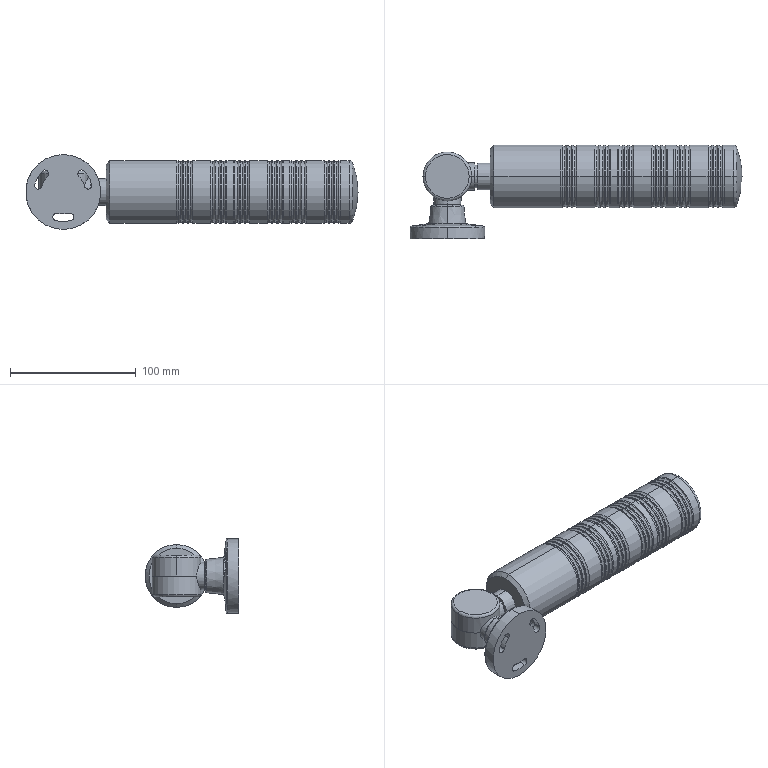Part | SolidWorks | 8 solids | 224 faces | box 263.704 x 74.5 x 59.5 mm | volume 261559 mm3 | cylinder 108 | torus 82 | plane 25 | cone 8 | sphere 1 | commonest cylinder face diameters 50 x50 6 x12 10 x12 38.7 x6 46 x6 21.9 x4